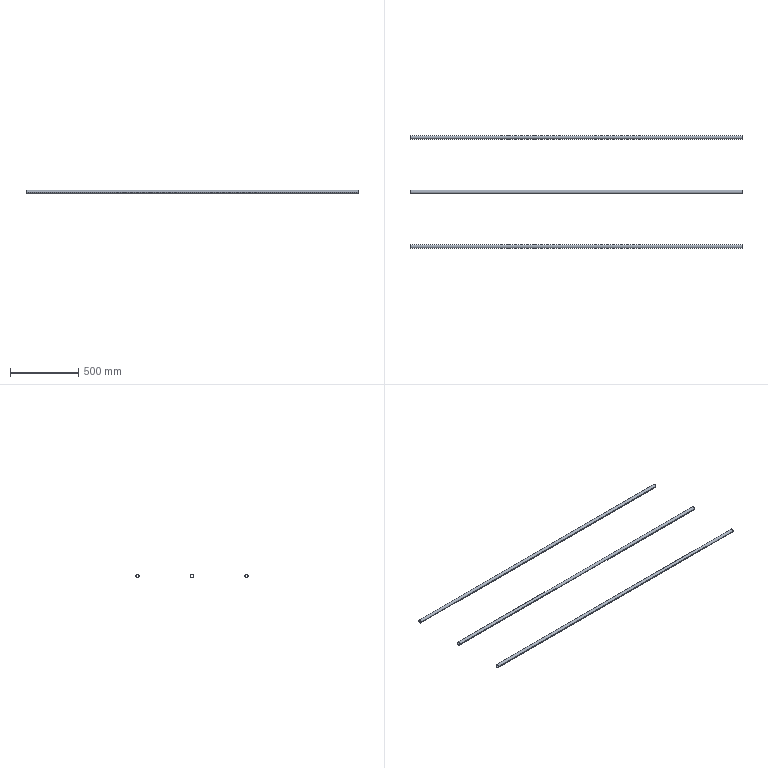Part | STEP file | 粉仓护栏栏杆4_Default<As Machined> | 3 solids | 18 faces | box 2430 x 825 x 25 mm | volume 807303 mm3 | cylinder 12 | plane 6 | commonest cylinder face diameters 22 x6 25 x6
STEP:
#1=CARTESIAN_POINT('',(0.,0.,0.));
#2=DIRECTION('',(0.,0.,1.));
#3=DIRECTION('',(1.,0.,0.));
#4=AXIS2_PLACEMENT_3D('',#1,#2,#3);
#5=CARTESIAN_POINT('',(1215.,812.5,0.));
#6=VERTEX_POINT('',#5);
#7=CARTESIAN_POINT('',(1215.,787.5,0.));
#8=VERTEX_POINT('',#7);
#9=CARTESIAN_POINT('',(1215.,800.,0.));
#10=DIRECTION('',(1.,0.,0.));
#11=DIRECTION('',(0.,1.,0.));
#12=AXIS2_PLACEMENT_3D('',#9,#10,#11);
#13=CIRCLE('',#12,12.5);
#14=CARTESIAN_POINT('',(1215.,800.,0.));
#15=DIRECTION('',(-1.,0.,0.));
#16=DIRECTION('',(0.,-1.,0.));
#17=AXIS2_PLACEMENT_3D('',#14,#15,#16);
#18=CYLINDRICAL_SURFACE('',#17,12.5);
#19=CARTESIAN_POINT('',(3.142,0.));
#20=DIRECTION('',(-1.,0.));
#21=VECTOR('',#20,1.);
#22=LINE('',#19,#21);
#23=(GEOMETRIC_REPRESENTATION_CONTEXT(2)PARAMETRIC_REPRESENTATION_CONTEXT()REPRESENTATION_CONTEXT('',''));
#24=DEFINITIONAL_REPRESENTATION('',(#22),#23);
#25=PCURVE('',#18,#24);
#26=CARTESIAN_POINT('',(1215.,800.,0.));
#27=DIRECTION('',(1.,0.,0.));
#28=DIRECTION('',(0.,1.,0.));
#29=AXIS2_PLACEMENT_3D('',#26,#27,#28);
#30=PLANE('',#29);
#31=CARTESIAN_POINT('',(0.,0.));
#32=DIRECTION('',(1.,0.));
#33=AXIS2_PLACEMENT_2D('',#31,#32);
#34=CIRCLE('',#33,12.5);
#35=(GEOMETRIC_REPRESENTATION_CONTEXT(2)PARAMETRIC_REPRESENTATION_CONTEXT()REPRESENTATION_CONTEXT('',''));
#36=DEFINITIONAL_REPRESENTATION('',(#34),#35);
#37=PCURVE('',#30,#36);
#38=SURFACE_CURVE('',#13,(#25,#37),.PCURVE_S1.);
#39=EDGE_CURVE('',#6,#8,#38,.T.);
#40=ORIENTED_EDGE('',*,*,#39,.F.);
#41=CARTESIAN_POINT('',(-1215.,812.5,0.));
#42=VERTEX_POINT('',#41);
#43=CARTESIAN_POINT('',(1215.,812.5,0.));
#44=DIRECTION('',(-1.,0.,0.));
#45=VECTOR('',#44,1.);
#46=LINE('',#43,#45);
#47=CARTESIAN_POINT('',(3.142,0.));
#48=DIRECTION('',(0.,1.));
#49=VECTOR('',#48,1.);
#50=LINE('',#47,#49);
#51=(GEOMETRIC_REPRESENTATION_CONTEXT(2)PARAMETRIC_REPRESENTATION_CONTEXT()REPRESENTATION_CONTEXT('',''));
#52=DEFINITIONAL_REPRESENTATION('',(#50),#51);
#53=PCURVE('',#18,#52);
#54=CARTESIAN_POINT('',(1215.,800.,0.));
#55=DIRECTION('',(-1.,0.,0.));
#56=DIRECTION('',(0.,-1.,0.));
#57=AXIS2_PLACEMENT_3D('',#54,#55,#56);
#58=CYLINDRICAL_SURFACE('',#57,12.5);
#59=CARTESIAN_POINT('',(3.142,0.));
#60=DIRECTION('',(0.,1.));
#61=VECTOR('',#60,1.);
#62=LINE('',#59,#61);
#63=(GEOMETRIC_REPRESENTATION_CONTEXT(2)PARAMETRIC_REPRESENTATION_CONTEXT()REPRESENTATION_CONTEXT('',''));
#64=DEFINITIONAL_REPRESENTATION('',(#62),#63);
#65=PCURVE('',#58,#64);
#66=SURFACE_CURVE('',#46,(#53,#65),.PCURVE_S1.);
#67=EDGE_CURVE('',#6,#42,#66,.T.);
#68=ORIENTED_EDGE('',*,*,#67,.T.);
#69=CARTESIAN_POINT('',(-1215.,787.5,0.));
#70=VERTEX_POINT('',#69);
#71=CARTESIAN_POINT('',(-1215.,800.,0.));
#72=DIRECTION('',(1.,0.,0.));
#73=DIRECTION('',(0.,1.,0.));
#74=AXIS2_PLACEMENT_3D('',#71,#72,#73);
#75=CIRCLE('',#74,12.5);
#76=CARTESIAN_POINT('',(3.142,2430.));
#77=DIRECTION('',(-1.,0.));
#78=VECTOR('',#77,1.);
#79=LINE('',#76,#78);
#80=(GEOMETRIC_REPRESENTATION_CONTEXT(2)PARAMETRIC_REPRESENTATION_CONTEXT()REPRESENTATION_CONTEXT('',''));
#81=DEFINITIONAL_REPRESENTATION('',(#79),#80);
#82=PCURVE('',#18,#81);
#83=CARTESIAN_POINT('',(-1215.,800.,0.));
#84=DIRECTION('',(1.,0.,0.));
#85=DIRECTION('',(0.,1.,0.));
#86=AXIS2_PLACEMENT_3D('',#83,#84,#85);
#87=PLANE('',#86);
#88=CARTESIAN_POINT('',(0.,0.));
#89=DIRECTION('',(1.,0.));
#90=AXIS2_PLACEMENT_2D('',#88,#89);
#91=CIRCLE('',#90,12.5);
#92=(GEOMETRIC_REPRESENTATION_CONTEXT(2)PARAMETRIC_REPRESENTATION_CONTEXT()REPRESENTATION_CONTEXT('',''));
#93=DEFINITIONAL_REPRESENTATION('',(#91),#92);
#94=PCURVE('',#87,#93);
#95=SURFACE_CURVE('',#75,(#82,#94),.PCURVE_S1.);
#96=EDGE_CURVE('',#42,#70,#95,.T.);
#97=ORIENTED_EDGE('',*,*,#96,.T.);
#98=CARTESIAN_POINT('',(1215.,787.5,0.));
#99=DIRECTION('',(-1.,0.,0.));
#100=VECTOR('',#99,1.);
#101=LINE('',#98,#100);
#102=CARTESIAN_POINT('',(0.,0.));
#103=DIRECTION('',(0.,1.));
#104=VECTOR('',#103,1.);
#105=LINE('',#102,#104);
#106=(GEOMETRIC_REPRESENTATION_CONTEXT(2)PARAMETRIC_REPRESENTATION_CONTEXT()REPRESENTATION_CONTEXT('',''));
#107=DEFINITIONAL_REPRESENTATION('',(#105),#106);
#108=PCURVE('',#18,#107);
#109=CARTESIAN_POINT('',(6.283,0.));
#110=DIRECTION('',(0.,1.));
#111=VECTOR('',#110,1.);
#112=LINE('',#109,#111);
#113=(GEOMETRIC_REPRESENTATION_CONTEXT(2)PARAMETRIC_REPRESENTATION_CONTEXT()REPRESENTATION_CONTEXT('',''));
#114=DEFINITIONAL_REPRESENTATION('',(#112),#113);
#115=PCURVE('',#58,#114);
#116=SURFACE_CURVE('',#101,(#108,#115),.PCURVE_S1.);
#117=EDGE_CURVE('',#8,#70,#116,.T.);
#118=ORIENTED_EDGE('',*,*,#117,.F.);
#119=EDGE_LOOP('',(#40,#68,#97,#118));
#120=FACE_BOUND('',#119,.T.);
#121=ADVANCED_FACE('',(#120),#18,.T.);
#122=CARTESIAN_POINT('',(1215.,789.,0.));
#123=VERTEX_POINT('',#122);
#124=CARTESIAN_POINT('',(-1215.,789.,0.));
#125=VERTEX_POINT('',#124);
#126=CARTESIAN_POINT('',(1215.,789.,0.));
#127=DIRECTION('',(-1.,0.,0.));
#128=VECTOR('',#127,1.);
#129=LINE('',#126,#128);
#130=CARTESIAN_POINT('',(1215.,800.,0.));
#131=DIRECTION('',(-1.,0.,0.));
#132=DIRECTION('',(0.,-1.,0.));
#133=AXIS2_PLACEMENT_3D('',#130,#131,#132);
#134=CYLINDRICAL_SURFACE('',#133,11.);
#135=CARTESIAN_POINT('',(6.283,0.));
#136=DIRECTION('',(0.,1.));
#137=VECTOR('',#136,1.);
#138=LINE('',#135,#137);
#139=(GEOMETRIC_REPRESENTATION_CONTEXT(2)PARAMETRIC_REPRESENTATION_CONTEXT()REPRESENTATION_CONTEXT('',''));
#140=DEFINITIONAL_REPRESENTATION('',(#138),#139);
#141=PCURVE('',#134,#140);
#142=CARTESIAN_POINT('',(1215.,800.,0.));
#143=DIRECTION('',(-1.,0.,0.));
#144=DIRECTION('',(0.,-1.,0.));
#145=AXIS2_PLACEMENT_3D('',#142,#143,#144);
#146=CYLINDRICAL_SURFACE('',#145,11.);
#147=CARTESIAN_POINT('',(0.,0.));
#148=DIRECTION('',(0.,1.));
#149=VECTOR('',#148,1.);
#150=LINE('',#147,#149);
#151=(GEOMETRIC_REPRESENTATION_CONTEXT(2)PARAMETRIC_REPRESENTATION_CONTEXT()REPRESENTATION_CONTEXT('',''));
#152=DEFINITIONAL_REPRESENTATION('',(#150),#151);
#153=PCURVE('',#146,#152);
#154=SURFACE_CURVE('',#129,(#141,#153),.PCURVE_S1.);
#155=EDGE_CURVE('',#123,#125,#154,.T.);
#156=ORIENTED_EDGE('',*,*,#155,.T.);
#157=CARTESIAN_POINT('',(-1215.,811.,0.));
#158=VERTEX_POINT('',#157);
#159=CARTESIAN_POINT('',(-1215.,800.,0.));
#160=DIRECTION('',(1.,0.,0.));
#161=DIRECTION('',(0.,1.,0.));
#162=AXIS2_PLACEMENT_3D('',#159,#160,#161);
#163=CIRCLE('',#162,11.);
#164=CARTESIAN_POINT('',(9.425,2430.));
#165=DIRECTION('',(-1.,0.));
#166=VECTOR('',#165,1.);
#167=LINE('',#164,#166);
#168=(GEOMETRIC_REPRESENTATION_CONTEXT(2)PARAMETRIC_REPRESENTATION_CONTEXT()REPRESENTATION_CONTEXT('',''));
#169=DEFINITIONAL_REPRESENTATION('',(#167),#168);
#170=PCURVE('',#134,#169);
#171=CARTESIAN_POINT('',(0.,0.));
#172=DIRECTION('',(1.,0.));
#173=AXIS2_PLACEMENT_2D('',#171,#172);
#174=CIRCLE('',#173,11.);
#175=(GEOMETRIC_REPRESENTATION_CONTEXT(2)PARAMETRIC_REPRESENTATION_CONTEXT()REPRESENTATION_CONTEXT('',''));
#176=DEFINITIONAL_REPRESENTATION('',(#174),#175);
#177=PCURVE('',#87,#176);
#178=SURFACE_CURVE('',#163,(#170,#177),.PCURVE_S1.);
#179=EDGE_CURVE('',#125,#158,#178,.T.);
#180=ORIENTED_EDGE('',*,*,#179,.T.);
#181=CARTESIAN_POINT('',(1215.,811.,0.));
#182=VERTEX_POINT('',#181);
#183=CARTESIAN_POINT('',(1215.,811.,0.));
#184=DIRECTION('',(-1.,0.,0.));
#185=VECTOR('',#184,1.);
#186=LINE('',#183,#185);
#187=CARTESIAN_POINT('',(3.142,0.));
#188=DIRECTION('',(0.,1.));
#189=VECTOR('',#188,1.);
#190=LINE('',#187,#189);
#191=(GEOMETRIC_REPRESENTATION_CONTEXT(2)PARAMETRIC_REPRESENTATION_CONTEXT()REPRESENTATION_CONTEXT('',''));
#192=DEFINITIONAL_REPRESENTATION('',(#190),#191);
#193=PCURVE('',#134,#192);
#194=CARTESIAN_POINT('',(3.142,0.));
#195=DIRECTION('',(0.,1.));
#196=VECTOR('',#195,1.);
#197=LINE('',#194,#196);
#198=(GEOMETRIC_REPRESENTATION_CONTEXT(2)PARAMETRIC_REPRESENTATION_CONTEXT()REPRESENTATION_CONTEXT('',''));
#199=DEFINITIONAL_REPRESENTATION('',(#197),#198);
#200=PCURVE('',#146,#199);
#201=SURFACE_CURVE('',#186,(#193,#200),.PCURVE_S1.);
#202=EDGE_CURVE('',#182,#158,#201,.T.);
#203=ORIENTED_EDGE('',*,*,#202,.F.);
#204=CARTESIAN_POINT('',(1215.,800.,0.));
#205=DIRECTION('',(1.,0.,0.));
#206=DIRECTION('',(0.,1.,0.));
#207=AXIS2_PLACEMENT_3D('',#204,#205,#206);
#208=CIRCLE('',#207,11.);
#209=CARTESIAN_POINT('',(9.425,0.));
#210=DIRECTION('',(-1.,0.));
#211=VECTOR('',#210,1.);
#212=LINE('',#209,#211);
#213=(GEOMETRIC_REPRESENTATION_CONTEXT(2)PARAMETRIC_REPRESENTATION_CONTEXT()REPRESENTATION_CONTEXT('',''));
#214=DEFINITIONAL_REPRESENTATION('',(#212),#213);
#215=PCURVE('',#134,#214);
#216=CARTESIAN_POINT('',(0.,0.));
#217=DIRECTION('',(1.,0.));
#218=AXIS2_PLACEMENT_2D('',#216,#217);
#219=CIRCLE('',#218,11.);
#220=(GEOMETRIC_REPRESENTATION_CONTEXT(2)PARAMETRIC_REPRESENTATION_CONTEXT()REPRESENTATION_CONTEXT('',''));
#221=DEFINITIONAL_REPRESENTATION('',(#219),#220);
#222=PCURVE('',#30,#221);
#223=SURFACE_CURVE('',#208,(#215,#222),.PCURVE_S1.);
#224=EDGE_CURVE('',#123,#182,#223,.T.);
#225=ORIENTED_EDGE('',*,*,#224,.F.);
#226=EDGE_LOOP('',(#156,#180,#203,#225));
#227=FACE_BOUND('',#226,.F.);
#228=ADVANCED_FACE('',(#227),#134,.F.);
#229=CARTESIAN_POINT('',(-1215.,800.,0.));
#230=DIRECTION('',(1.,0.,0.));
#231=DIRECTION('',(0.,1.,0.));
#232=AXIS2_PLACEMENT_3D('',#229,#230,#231);
#233=CIRCLE('',#232,11.);
#234=CARTESIAN_POINT('',(3.142,2430.));
#235=DIRECTION('',(-1.,0.));
#236=VECTOR('',#235,1.);
#237=LINE('',#234,#236);
#238=(GEOMETRIC_REPRESENTATION_CONTEXT(2)PARAMETRIC_REPRESENTATION_CONTEXT()REPRESENTATION_CONTEXT('',''));
#239=DEFINITIONAL_REPRESENTATION('',(#237),#238);
#240=PCURVE('',#146,#239);
#241=CARTESIAN_POINT('',(0.,0.));
#242=DIRECTION('',(1.,0.));
#243=AXIS2_PLACEMENT_2D('',#241,#242);
#244=CIRCLE('',#243,11.);
#245=(GEOMETRIC_REPRESENTATION_CONTEXT(2)PARAMETRIC_REPRESENTATION_CONTEXT()REPRESENTATION_CONTEXT('',''));
#246=DEFINITIONAL_REPRESENTATION('',(#244),#245);
#247=PCURVE('',#87,#246);
#248=SURFACE_CURVE('',#233,(#240,#247),.PCURVE_S1.);
#249=EDGE_CURVE('',#158,#125,#248,.T.);
#250=ORIENTED_EDGE('',*,*,#249,.T.);
#251=ORIENTED_EDGE('',*,*,#155,.F.);
#252=CARTESIAN_POINT('',(1215.,800.,0.));
#253=DIRECTION('',(1.,0.,0.));
#254=DIRECTION('',(0.,1.,0.));
#255=AXIS2_PLACEMENT_3D('',#252,#253,#254);
#256=CIRCLE('',#255,11.);
#257=CARTESIAN_POINT('',(3.142,0.));
#258=DIRECTION('',(-1.,0.));
#259=VECTOR('',#258,1.);
#260=LINE('',#257,#259);
#261=(GEOMETRIC_REPRESENTATION_CONTEXT(2)PARAMETRIC_REPRESENTATION_CONTEXT()REPRESENTATION_CONTEXT('',''));
#262=DEFINITIONAL_REPRESENTATION('',(#260),#261);
#263=PCURVE('',#146,#262);
#264=CARTESIAN_POINT('',(0.,0.));
#265=DIRECTION('',(1.,0.));
#266=AXIS2_PLACEMENT_2D('',#264,#265);
#267=CIRCLE('',#266,11.);
#268=(GEOMETRIC_REPRESENTATION_CONTEXT(2)PARAMETRIC_REPRESENTATION_CONTEXT()REPRESENTATION_CONTEXT('',''));
#269=DEFINITIONAL_REPRESENTATION('',(#267),#268);
#270=PCURVE('',#30,#269);
#271=SURFACE_CURVE('',#256,(#263,#270),.PCURVE_S1.);
#272=EDGE_CURVE('',#182,#123,#271,.T.);
#273=ORIENTED_EDGE('',*,*,#272,.F.);
#274=ORIENTED_EDGE('',*,*,#202,.T.);
#275=EDGE_LOOP('',(#250,#251,#273,#274));
#276=FACE_BOUND('',#275,.F.);
#277=ADVANCED_FACE('',(#276),#146,.F.);
#278=ORIENTED_EDGE('',*,*,#67,.F.);
#279=CARTESIAN_POINT('',(1215.,800.,0.));
#280=DIRECTION('',(1.,0.,0.));
#281=DIRECTION('',(0.,1.,0.));
#282=AXIS2_PLACEMENT_3D('',#279,#280,#281);
#283=CIRCLE('',#282,12.5);
#284=CARTESIAN_POINT('',(9.425,0.));
#285=DIRECTION('',(-1.,0.));
#286=VECTOR('',#285,1.);
#287=LINE('',#284,#286);
#288=(GEOMETRIC_REPRESENTATION_CONTEXT(2)PARAMETRIC_REPRESENTATION_CONTEXT()REPRESENTATION_CONTEXT('',''));
#289=DEFINITIONAL_REPRESENTATION('',(#287),#288);
#290=PCURVE('',#58,#289);
#291=CARTESIAN_POINT('',(0.,0.));
#292=DIRECTION('',(1.,0.));
#293=AXIS2_PLACEMENT_2D('',#291,#292);
#294=CIRCLE('',#293,12.5);
#295=(GEOMETRIC_REPRESENTATION_CONTEXT(2)PARAMETRIC_REPRESENTATION_CONTEXT()REPRESENTATION_CONTEXT('',''));
#296=DEFINITIONAL_REPRESENTATION('',(#294),#295);
#297=PCURVE('',#30,#296);
#298=SURFACE_CURVE('',#283,(#290,#297),.PCURVE_S1.);
#299=EDGE_CURVE('',#8,#6,#298,.T.);
#300=ORIENTED_EDGE('',*,*,#299,.F.);
#301=ORIENTED_EDGE('',*,*,#117,.T.);
#302=CARTESIAN_POINT('',(-1215.,800.,0.));
#303=DIRECTION('',(1.,0.,0.));
#304=DIRECTION('',(0.,1.,0.));
#305=AXIS2_PLACEMENT_3D('',#302,#303,#304);
#306=CIRCLE('',#305,12.5);
#307=CARTESIAN_POINT('',(9.425,2430.));
#308=DIRECTION('',(-1.,0.));
#309=VECTOR('',#308,1.);
#310=LINE('',#307,#309);
#311=(GEOMETRIC_REPRESENTATION_CONTEXT(2)PARAMETRIC_REPRESENTATION_CONTEXT()REPRESENTATION_CONTEXT('',''));
#312=DEFINITIONAL_REPRESENTATION('',(#310),#311);
#313=PCURVE('',#58,#312);
#314=CARTESIAN_POINT('',(0.,0.));
#315=DIRECTION('',(1.,0.));
#316=AXIS2_PLACEMENT_2D('',#314,#315);
#317=CIRCLE('',#316,12.5);
#318=(GEOMETRIC_REPRESENTATION_CONTEXT(2)PARAMETRIC_REPRESENTATION_CONTEXT()REPRESENTATION_CONTEXT('',''));
#319=DEFINITIONAL_REPRESENTATION('',(#317),#318);
#320=PCURVE('',#87,#319);
#321=SURFACE_CURVE('',#306,(#313,#320),.PCURVE_S1.);
#322=EDGE_CURVE('',#70,#42,#321,.T.);
#323=ORIENTED_EDGE('',*,*,#322,.T.);
#324=EDGE_LOOP('',(#278,#300,#301,#323));
#325=FACE_BOUND('',#324,.T.);
#326=ADVANCED_FACE('',(#325),#58,.T.);
#327=ORIENTED_EDGE('',*,*,#224,.F.);
#328=ORIENTED_EDGE('',*,*,#272,.F.);
#329=EDGE_LOOP('',(#327,#328));
#330=FACE_BOUND('',#329,.T.);
#331=ORIENTED_EDGE('',*,*,#299,.T.);
#332=ORIENTED_EDGE('',*,*,#39,.T.);
#333=EDGE_LOOP('',(#331,#332));
#334=FACE_BOUND('',#333,.T.);
#335=ADVANCED_FACE('',(#330,#334),#30,.T.);
#336=ORIENTED_EDGE('',*,*,#179,.T.);
#337=ORIENTED_EDGE('',*,*,#249,.T.);
#338=EDGE_LOOP('',(#336,#337));
#339=FACE_BOUND('',#338,.T.);
#340=ORIENTED_EDGE('',*,*,#322,.F.);
#341=ORIENTED_EDGE('',*,*,#96,.F.);
#342=EDGE_LOOP('',(#340,#341));
#343=FACE_BOUND('',#342,.T.);
#344=ADVANCED_FACE('',(#339,#343),#87,.F.);
#345=CLOSED_SHELL('',(#121,#228,#277,#326,#335,#344));
#346=MANIFOLD_SOLID_BREP('',#345);
#347=CARTESIAN_POINT('',(1215.,12.5,0.));
#348=VERTEX_POINT('',#347);
#349=CARTESIAN_POINT('',(1215.,-12.5,0.));
#350=VERTEX_POINT('',#349);
#351=CARTESIAN_POINT('',(1215.,0.,0.));
#352=DIRECTION('',(1.,0.,0.));
#353=DIRECTION('',(0.,1.,0.));
#354=AXIS2_PLACEMENT_3D('',#351,#352,#353);
#355=CIRCLE('',#354,12.5);
#356=CARTESIAN_POINT('',(1215.,0.,0.));
#357=DIRECTION('',(-1.,0.,0.));
#358=DIRECTION('',(0.,-1.,0.));
#359=AXIS2_PLACEMENT_3D('',#356,#357,#358);
#360=CYLINDRICAL_SURFACE('',#359,12.5);
#361=CARTESIAN_POINT('',(3.142,0.));
#362=DIRECTION('',(-1.,0.));
#363=VECTOR('',#362,1.);
#364=LINE('',#361,#363);
#365=(GEOMETRIC_REPRESENTATION_CONTEXT(2)PARAMETRIC_REPRESENTATION_CONTEXT()REPRESENTATION_CONTEXT('',''));
#366=DEFINITIONAL_REPRESENTATION('',(#364),#365);
#367=PCURVE('',#360,#366);
#368=CARTESIAN_POINT('',(1215.,0.,0.));
#369=DIRECTION('',(1.,0.,0.));
#370=DIRECTION('',(0.,1.,0.));
#371=AXIS2_PLACEMENT_3D('',#368,#369,#370);
#372=PLANE('',#371);
#373=CARTESIAN_POINT('',(0.,0.));
#374=DIRECTION('',(1.,0.));
#375=AXIS2_PLACEMENT_2D('',#373,#374);
#376=CIRCLE('',#375,12.5);
#377=(GEOMETRIC_REPRESENTATION_CONTEXT(2)PARAMETRIC_REPRESENTATION_CONTEXT()REPRESENTATION_CONTEXT('',''));
#378=DEFINITIONAL_REPRESENTATION('',(#376),#377);
#379=PCURVE('',#372,#378);
#380=SURFACE_CURVE('',#355,(#367,#379),.PCURVE_S1.);
#381=EDGE_CURVE('',#348,#350,#380,.T.);
#382=ORIENTED_EDGE('',*,*,#381,.F.);
#383=CARTESIAN_POINT('',(-1215.,12.5,0.));
#384=VERTEX_POINT('',#383);
#385=CARTESIAN_POINT('',(1215.,12.5,0.));
#386=DIRECTION('',(-1.,0.,0.));
#387=VECTOR('',#386,1.);
#388=LINE('',#385,#387);
#389=CARTESIAN_POINT('',(3.142,0.));
#390=DIRECTION('',(0.,1.));
#391=VECTOR('',#390,1.);
#392=LINE('',#389,#391);
#393=(GEOMETRIC_REPRESENTATION_CONTEXT(2)PARAMETRIC_REPRESENTATION_CONTEXT()REPRESENTATION_CONTEXT('',''));
#394=DEFINITIONAL_REPRESENTATION('',(#392),#393);
#395=PCURVE('',#360,#394);
#396=CARTESIAN_POINT('',(1215.,0.,0.));
#397=DIRECTION('',(-1.,0.,0.));
#398=DIRECTION('',(0.,-1.,0.));
#399=AXIS2_PLACEMENT_3D('',#396,#397,#398);
#400=CYLINDRICAL_SURFACE('',#399,12.5);
#401=CARTESIAN_POINT('',(3.142,0.));
#402=DIRECTION('',(0.,1.));
#403=VECTOR('',#402,1.);
#404=LINE('',#401,#403);
#405=(GEOMETRIC_REPRESENTATION_CONTEXT(2)PARAMETRIC_REPRESENTATION_CONTEXT()REPRESENTATION_CONTEXT('',''));
#406=DEFINITIONAL_REPRESENTATION('',(#404),#405);
#407=PCURVE('',#400,#406);
#408=SURFACE_CURVE('',#388,(#395,#407),.PCURVE_S1.);
#409=EDGE_CURVE('',#348,#384,#408,.T.);
#410=ORIENTED_EDGE('',*,*,#409,.T.);
#411=CARTESIAN_POINT('',(-1215.,-12.5,0.));
#412=VERTEX_POINT('',#411);
#413=CARTESIAN_POINT('',(-1215.,0.,0.));
#414=DIRECTION('',(1.,0.,0.));
#415=DIRECTION('',(0.,1.,0.));
#416=AXIS2_PLACEMENT_3D('',#413,#414,#415);
#417=CIRCLE('',#416,12.5);
#418=CARTESIAN_POINT('',(3.142,2430.));
#419=DIRECTION('',(-1.,0.));
#420=VECTOR('',#419,1.);
#421=LINE('',#418,#420);
#422=(GEOMETRIC_REPRESENTATION_CONTEXT(2)PARAMETRIC_REPRESENTATION_CONTEXT()REPRESENTATION_CONTEXT('',''));
#423=DEFINITIONAL_REPRESENTATION('',(#421),#422);
#424=PCURVE('',#360,#423);
#425=CARTESIAN_POINT('',(-1215.,0.,0.));
#426=DIRECTION('',(1.,0.,0.));
#427=DIRECTION('',(0.,1.,0.));
#428=AXIS2_PLACEMENT_3D('',#425,#426,#427);
#429=PLANE('',#428);
#430=CARTESIAN_POINT('',(0.,0.));
#431=DIRECTION('',(1.,0.));
#432=AXIS2_PLACEMENT_2D('',#430,#431);
#433=CIRCLE('',#432,12.5);
#434=(GEOMETRIC_REPRESENTATION_CONTEXT(2)PARAMETRIC_REPRESENTATION_CONTEXT()REPRESENTATION_CONTEXT('',''));
#435=DEFINITIONAL_REPRESENTATION('',(#433),#434);
#436=PCURVE('',#429,#435);
#437=SURFACE_CURVE('',#417,(#424,#436),.PCURVE_S1.);
#438=EDGE_CURVE('',#384,#412,#437,.T.);
#439=ORIENTED_EDGE('',*,*,#438,.T.);
#440=CARTESIAN_POINT('',(1215.,-12.5,0.));
#441=DIRECTION('',(-1.,0.,0.));
#442=VECTOR('',#441,1.);
#443=LINE('',#440,#442);
#444=CARTESIAN_POINT('',(0.,0.));
#445=DIRECTION('',(0.,1.));
#446=VECTOR('',#445,1.);
#447=LINE('',#444,#446);
#448=(GEOMETRIC_REPRESENTATION_CONTEXT(2)PARAMETRIC_REPRESENTATION_CONTEXT()REPRESENTATION_CONTEXT('',''));
#449=DEFINITIONAL_REPRESENTATION('',(#447),#448);
#450=PCURVE('',#360,#449);
#451=CARTESIAN_POINT('',(6.283,0.));
#452=DIRECTION('',(0.,1.));
#453=VECTOR('',#452,1.);
#454=LINE('',#451,#453);
#455=(GEOMETRIC_REPRESENTATION_CONTEXT(2)PARAMETRIC_REPRESENTATION_CONTEXT()REPRESENTATION_CONTEXT('',''));
#456=DEFINITIONAL_REPRESENTATION('',(#454),#455);
#457=PCURVE('',#400,#456);
#458=SURFACE_CURVE('',#443,(#450,#457),.PCURVE_S1.);
#459=EDGE_CURVE('',#350,#412,#458,.T.);
#460=ORIENTED_EDGE('',*,*,#459,.F.);
#461=EDGE_LOOP('',(#382,#410,#439,#460));
#462=FACE_BOUND('',#461,.T.);
#463=ADVANCED_FACE('',(#462),#360,.T.);
#464=CARTESIAN_POINT('',(1215.,-11.,0.));
#465=VERTEX_POINT('',#464);
#466=CARTESIAN_POINT('',(-1215.,-11.,0.));
#467=VERTEX_POINT('',#466);
#468=CARTESIAN_POINT('',(1215.,-11.,0.));
#469=DIRECTION('',(-1.,0.,0.));
#470=VECTOR('',#469,1.);
#471=LINE('',#468,#470);
#472=CARTESIAN_POINT('',(1215.,0.,0.));
#473=DIRECTION('',(-1.,0.,0.));
#474=DIRECTION('',(0.,-1.,0.));
#475=AXIS2_PLACEMENT_3D('',#472,#473,#474);
#476=CYLINDRICAL_SURFACE('',#475,11.);
#477=CARTESIAN_POINT('',(6.283,0.));
#478=DIRECTION('',(0.,1.));
#479=VECTOR('',#478,1.);
#480=LINE('',#477,#479);
#481=(GEOMETRIC_REPRESENTATION_CONTEXT(2)PARAMETRIC_REPRESENTATION_CONTEXT()REPRESENTATION_CONTEXT('',''));
#482=DEFINITIONAL_REPRESENTATION('',(#480),#481);
#483=PCURVE('',#476,#482);
#484=CARTESIAN_POINT('',(1215.,0.,0.));
#485=DIRECTION('',(-1.,0.,0.));
#486=DIRECTION('',(0.,-1.,0.));
#487=AXIS2_PLACEMENT_3D('',#484,#485,#486);
#488=CYLINDRICAL_SURFACE('',#487,11.);
#489=CARTESIAN_POINT('',(0.,0.));
#490=DIRECTION('',(0.,1.));
#491=VECTOR('',#490,1.);
#492=LINE('',#489,#491);
#493=(GEOMETRIC_REPRESENTATION_CONTEXT(2)PARAMETRIC_REPRESENTATION_CONTEXT()REPRESENTATION_CONTEXT('',''));
#494=DEFINITIONAL_REPRESENTATION('',(#492),#493);
#495=PCURVE('',#488,#494);
#496=SURFACE_CURVE('',#471,(#483,#495),.PCURVE_S1.);
#497=EDGE_CURVE('',#465,#467,#496,.T.);
#498=ORIENTED_EDGE('',*,*,#497,.T.);
#499=CARTESIAN_POINT('',(-1215.,11.,0.));
#500=VERTEX_POINT('',#499);
#501=CARTESIAN_POINT('',(-1215.,0.,0.));
#502=DIRECTION('',(1.,0.,0.));
#503=DIRECTION('',(0.,1.,0.));
#504=AXIS2_PLACEMENT_3D('',#501,#502,#503);
#505=CIRCLE('',#504,11.);
#506=CARTESIAN_POINT('',(9.425,2430.));
#507=DIRECTION('',(-1.,0.));
#508=VECTOR('',#507,1.);
#509=LINE('',#506,#508);
#510=(GEOMETRIC_REPRESENTATION_CONTEXT(2)PARAMETRIC_REPRESENTATION_CONTEXT()REPRESENTATION_CONTEXT('',''));
#511=DEFINITIONAL_REPRESENTATION('',(#509),#510);
#512=PCURVE('',#476,#511);
#513=CARTESIAN_POINT('',(0.,0.));
#514=DIRECTION('',(1.,0.));
#515=AXIS2_PLACEMENT_2D('',#513,#514);
#516=CIRCLE('',#515,11.);
#517=(GEOMETRIC_REPRESENTATION_CONTEXT(2)PARAMETRIC_REPRESENTATION_CONTEXT()REPRESENTATION_CONTEXT('',''));
#518=DEFINITIONAL_REPRESENTATION('',(#516),#517);
#519=PCURVE('',#429,#518);
#520=SURFACE_CURVE('',#505,(#512,#519),.PCURVE_S1.);
#521=EDGE_CURVE('',#467,#500,#520,.T.);
#522=ORIENTED_EDGE('',*,*,#521,.T.);
#523=CARTESIAN_POINT('',(1215.,11.,0.));
#524=VERTEX_POINT('',#523);
#525=CARTESIAN_POINT('',(1215.,11.,0.));
#526=DIRECTION('',(-1.,0.,0.));
#527=VECTOR('',#526,1.);
#528=LINE('',#525,#527);
#529=CARTESIAN_POINT('',(3.142,0.));
#530=DIRECTION('',(0.,1.));
#531=VECTOR('',#530,1.);
#532=LINE('',#529,#531);
#533=(GEOMETRIC_REPRESENTATION_CONTEXT(2)PARAMETRIC_REPRESENTATION_CONTEXT()REPRESENTATION_CONTEXT('',''));
#534=DEFINITIONAL_REPRESENTATION('',(#532),#533);
#535=PCURVE('',#476,#534);
#536=CARTESIAN_POINT('',(3.142,0.));
#537=DIRECTION('',(0.,1.));
#538=VECTOR('',#537,1.);
#539=LINE('',#536,#538);
#540=(GEOMETRIC_REPRESENTATION_CONTEXT(2)PARAMETRIC_REPRESENTATION_CONTEXT()REPRESENTATION_CONTEXT('',''));
#541=DEFINITIONAL_REPRESENTATION('',(#539),#540);
#542=PCURVE('',#488,#541);
#543=SURFACE_CURVE('',#528,(#535,#542),.PCURVE_S1.);
#544=EDGE_CURVE('',#524,#500,#543,.T.);
#545=ORIENTED_EDGE('',*,*,#544,.F.);
#546=CARTESIAN_POINT('',(1215.,0.,0.));
#547=DIRECTION('',(1.,0.,0.));
#548=DIRECTION('',(0.,1.,0.));
#549=AXIS2_PLACEMENT_3D('',#546,#547,#548);
#550=CIRCLE('',#549,11.);
#551=CARTESIAN_POINT('',(9.425,0.));
#552=DIRECTION('',(-1.,0.));
#553=VECTOR('',#552,1.);
#554=LINE('',#551,#553);
#555=(GEOMETRIC_REPRESENTATION_CONTEXT(2)PARAMETRIC_REPRESENTATION_CONTEXT()REPRESENTATION_CONTEXT('',''));
#556=DEFINITIONAL_REPRESENTATION('',(#554),#555);
#557=PCURVE('',#476,#556);
#558=CARTESIAN_POINT('',(0.,0.));
#559=DIRECTION('',(1.,0.));
#560=AXIS2_PLACEMENT_2D('',#558,#559);
#561=CIRCLE('',#560,11.);
#562=(GEOMETRIC_REPRESENTATION_CONTEXT(2)PARAMETRIC_REPRESENTATION_CONTEXT()REPRESENTATION_CONTEXT('',''));
#563=DEFINITIONAL_REPRESENTATION('',(#561),#562);
#564=PCURVE('',#372,#563);
#565=SURFACE_CURVE('',#550,(#557,#564),.PCURVE_S1.);
#566=EDGE_CURVE('',#465,#524,#565,.T.);
#567=ORIENTED_EDGE('',*,*,#566,.F.);
#568=EDGE_LOOP('',(#498,#522,#545,#567));
#569=FACE_BOUND('',#568,.F.);
#570=ADVANCED_FACE('',(#569),#476,.F.);
#571=CARTESIAN_POINT('',(-1215.,0.,0.));
#572=DIRECTION('',(1.,0.,0.));
#573=DIRECTION('',(0.,1.,0.));
#574=AXIS2_PLACEMENT_3D('',#571,#572,#573);
#575=CIRCLE('',#574,11.);
#576=CARTESIAN_POINT('',(3.142,2430.));
#577=DIRECTION('',(-1.,0.));
#578=VECTOR('',#577,1.);
#579=LINE('',#576,#578);
#580=(GEOMETRIC_REPRESENTATION_CONTEXT(2)PARAMETRIC_REPRESENTATION_CONTEXT()REPRESENTATION_CONTEXT('',''));
#581=DEFINITIONAL_REPRESENTATION('',(#579),#580);
#582=PCURVE('',#488,#581);
#583=CARTESIAN_POINT('',(0.,0.));
#584=DIRECTION('',(1.,0.));
#585=AXIS2_PLACEMENT_2D('',#583,#584);
#586=CIRCLE('',#585,11.);
#587=(GEOMETRIC_REPRESENTATION_CONTEXT(2)PARAMETRIC_REPRESENTATION_CONTEXT()REPRESENTATION_CONTEXT('',''));
#588=DEFINITIONAL_REPRESENTATION('',(#586),#587);
#589=PCURVE('',#429,#588);
#590=SURFACE_CURVE('',#575,(#582,#589),.PCURVE_S1.);
#591=EDGE_CURVE('',#500,#467,#590,.T.);
#592=ORIENTED_EDGE('',*,*,#591,.T.);
#593=ORIENTED_EDGE('',*,*,#497,.F.);
#594=CARTESIAN_POINT('',(1215.,0.,0.));
#595=DIRECTION('',(1.,0.,0.));
#596=DIRECTION('',(0.,1.,0.));
#597=AXIS2_PLACEMENT_3D('',#594,#595,#596);
#598=CIRCLE('',#597,11.);
#599=CARTESIAN_POINT('',(3.142,0.));
#600=DIRECTION('',(-1.,0.));
#601=VECTOR('',#600,1.);
#602=LINE('',#599,#601);
#603=(GEOMETRIC_REPRESENTATION_CONTEXT(2)PARAMETRIC_REPRESENTATION_CONTEXT()REPRESENTATION_CONTEXT('',''));
#604=DEFINITIONAL_REPRESENTATION('',(#602),#603);
#605=PCURVE('',#488,#604);
#606=CARTESIAN_POINT('',(0.,0.));
#607=DIRECTION('',(1.,0.));
#608=AXIS2_PLACEMENT_2D('',#606,#607);
#609=CIRCLE('',#608,11.);
#610=(GEOMETRIC_REPRESENTATION_CONTEXT(2)PARAMETRIC_REPRESENTATION_CONTEXT()REPRESENTATION_CONTEXT('',''));
#611=DEFINITIONAL_REPRESENTATION('',(#609),#610);
#612=PCURVE('',#372,#611);
#613=SURFACE_CURVE('',#598,(#605,#612),.PCURVE_S1.);
#614=EDGE_CURVE('',#524,#465,#613,.T.);
#615=ORIENTED_EDGE('',*,*,#614,.F.);
#616=ORIENTED_EDGE('',*,*,#544,.T.);
#617=EDGE_LOOP('',(#592,#593,#615,#616));
#618=FACE_BOUND('',#617,.F.);
#619=ADVANCED_FACE('',(#618),#488,.F.);
#620=ORIENTED_EDGE('',*,*,#409,.F.);
#621=CARTESIAN_POINT('',(1215.,0.,0.));
#622=DIRECTION('',(1.,0.,0.));
#623=DIRECTION('',(0.,1.,0.));
#624=AXIS2_PLACEMENT_3D('',#621,#622,#623);
#625=CIRCLE('',#624,12.5);
#626=CARTESIAN_POINT('',(9.425,0.));
#627=DIRECTION('',(-1.,0.));
#628=VECTOR('',#627,1.);
#629=LINE('',#626,#628);
#630=(GEOMETRIC_REPRESENTATION_CONTEXT(2)PARAMETRIC_REPRESENTATION_CONTEXT()REPRESENTATION_CONTEXT('',''));
#631=DEFINITIONAL_REPRESENTATION('',(#629),#630);
#632=PCURVE('',#400,#631);
#633=CARTESIAN_POINT('',(0.,0.));
#634=DIRECTION('',(1.,0.));
#635=AXIS2_PLACEMENT_2D('',#633,#634);
#636=CIRCLE('',#635,12.5);
#637=(GEOMETRIC_REPRESENTATION_CONTEXT(2)PARAMETRIC_REPRESENTATION_CONTEXT()REPRESENTATION_CONTEXT('',''));
#638=DEFINITIONAL_REPRESENTATION('',(#636),#637);
#639=PCURVE('',#372,#638);
#640=SURFACE_CURVE('',#625,(#632,#639),.PCURVE_S1.);
#641=EDGE_CURVE('',#350,#348,#640,.T.);
#642=ORIENTED_EDGE('',*,*,#641,.F.);
#643=ORIENTED_EDGE('',*,*,#459,.T.);
#644=CARTESIAN_POINT('',(-1215.,0.,0.));
#645=DIRECTION('',(1.,0.,0.));
#646=DIRECTION('',(0.,1.,0.));
#647=AXIS2_PLACEMENT_3D('',#644,#645,#646);
#648=CIRCLE('',#647,12.5);
#649=CARTESIAN_POINT('',(9.425,2430.));
#650=DIRECTION('',(-1.,0.));
#651=VECTOR('',#650,1.);
#652=LINE('',#649,#651);
#653=(GEOMETRIC_REPRESENTATION_CONTEXT(2)PARAMETRIC_REPRESENTATION_CONTEXT()REPRESENTATION_CONTEXT('',''));
#654=DEFINITIONAL_REPRESENTATION('',(#652),#653);
#655=PCURVE('',#400,#654);
#656=CARTESIAN_POINT('',(0.,0.));
#657=DIRECTION('',(1.,0.));
#658=AXIS2_PLACEMENT_2D('',#656,#657);
#659=CIRCLE('',#658,12.5);
#660=(GEOMETRIC_REPRESENTATION_CONTEXT(2)PARAMETRIC_REPRESENTATION_CONTEXT()REPRESENTATION_CONTEXT('',''));
#661=DEFINITIONAL_REPRESENTATION('',(#659),#660);
#662=PCURVE('',#429,#661);
#663=SURFACE_CURVE('',#648,(#655,#662),.PCURVE_S1.);
#664=EDGE_CURVE('',#412,#384,#663,.T.);
#665=ORIENTED_EDGE('',*,*,#664,.T.);
#666=EDGE_LOOP('',(#620,#642,#643,#665));
#667=FACE_BOUND('',#666,.T.);
#668=ADVANCED_FACE('',(#667),#400,.T.);
#669=ORIENTED_EDGE('',*,*,#566,.F.);
#670=ORIENTED_EDGE('',*,*,#614,.F.);
#671=EDGE_LOOP('',(#669,#670));
#672=FACE_BOUND('',#671,.T.);
#673=ORIENTED_EDGE('',*,*,#641,.T.);
#674=ORIENTED_EDGE('',*,*,#381,.T.);
#675=EDGE_LOOP('',(#673,#674));
#676=FACE_BOUND('',#675,.T.);
#677=ADVANCED_FACE('',(#672,#676),#372,.T.);
#678=ORIENTED_EDGE('',*,*,#521,.T.);
#679=ORIENTED_EDGE('',*,*,#591,.T.);
#680=EDGE_LOOP('',(#678,#679));
#681=FACE_BOUND('',#680,.T.);
#682=ORIENTED_EDGE('',*,*,#664,.F.);
#683=ORIENTED_EDGE('',*,*,#438,.F.);
#684=EDGE_LOOP('',(#682,#683));
#685=FACE_BOUND('',#684,.T.);
#686=ADVANCED_FACE('',(#681,#685),#429,.F.);
#687=CLOSED_SHELL('',(#463,#570,#619,#668,#677,#686));
#688=MANIFOLD_SOLID_BREP('',#687);
#689=CARTESIAN_POINT('',(1215.,412.5,0.));
#690=VERTEX_POINT('',#689);
#691=CARTESIAN_POINT('',(1215.,387.5,0.));
#692=VERTEX_POINT('',#691);
#693=CARTESIAN_POINT('',(1215.,400.,0.));
#694=DIRECTION('',(1.,0.,0.));
#695=DIRECTION('',(0.,1.,0.));
#696=AXIS2_PLACEMENT_3D('',#693,#694,#695);
#697=CIRCLE('',#696,12.5);
#698=CARTESIAN_POINT('',(1215.,400.,0.));
#699=DIRECTION('',(-1.,0.,0.));
#700=DIRECTION('',(0.,-1.,0.));
#701=AXIS2_PLACEMENT_3D('',#698,#699,#700);
#702=CYLINDRICAL_SURFACE('',#701,12.5);
#703=CARTESIAN_POINT('',(3.142,0.));
#704=DIRECTION('',(-1.,0.));
#705=VECTOR('',#704,1.);
#706=LINE('',#703,#705);
#707=(GEOMETRIC_REPRESENTATION_CONTEXT(2)PARAMETRIC_REPRESENTATION_CONTEXT()REPRESENTATION_CONTEXT('',''));
#708=DEFINITIONAL_REPRESENTATION('',(#706),#707);
#709=PCURVE('',#702,#708);
#710=CARTESIAN_POINT('',(1215.,400.,0.));
#711=DIRECTION('',(1.,0.,0.));
#712=DIRECTION('',(0.,1.,0.));
#713=AXIS2_PLACEMENT_3D('',#710,#711,#712);
#714=PLANE('',#713);
#715=CARTESIAN_POINT('',(0.,0.));
#716=DIRECTION('',(1.,0.));
#717=AXIS2_PLACEMENT_2D('',#715,#716);
#718=CIRCLE('',#717,12.5);
#719=(GEOMETRIC_REPRESENTATION_CONTEXT(2)PARAMETRIC_REPRESENTATION_CONTEXT()REPRESENTATION_CONTEXT('',''));
#720=DEFINITIONAL_REPRESENTATION('',(#718),#719);
#721=PCURVE('',#714,#720);
#722=SURFACE_CURVE('',#697,(#709,#721),.PCURVE_S1.);
#723=EDGE_CURVE('',#690,#692,#722,.T.);
#724=ORIENTED_EDGE('',*,*,#723,.F.);
#725=CARTESIAN_POINT('',(-1215.,412.5,0.));
#726=VERTEX_POINT('',#725);
#727=CARTESIAN_POINT('',(1215.,412.5,0.));
#728=DIRECTION('',(-1.,0.,0.));
#729=VECTOR('',#728,1.);
#730=LINE('',#727,#729);
#731=CARTESIAN_POINT('',(3.142,0.));
#732=DIRECTION('',(0.,1.));
#733=VECTOR('',#732,1.);
#734=LINE('',#731,#733);
#735=(GEOMETRIC_REPRESENTATION_CONTEXT(2)PARAMETRIC_REPRESENTATION_CONTEXT()REPRESENTATION_CONTEXT('',''));
#736=DEFINITIONAL_REPRESENTATION('',(#734),#735);
#737=PCURVE('',#702,#736);
#738=CARTESIAN_POINT('',(1215.,400.,0.));
#739=DIRECTION('',(-1.,0.,0.));
#740=DIRECTION('',(0.,-1.,0.));
#741=AXIS2_PLACEMENT_3D('',#738,#739,#740);
#742=CYLINDRICAL_SURFACE('',#741,12.5);
#743=CARTESIAN_POINT('',(3.142,0.));
#744=DIRECTION('',(0.,1.));
#745=VECTOR('',#744,1.);
#746=LINE('',#743,#745);
#747=(GEOMETRIC_REPRESENTATION_CONTEXT(2)PARAMETRIC_REPRESENTATION_CONTEXT()REPRESENTATION_CONTEXT('',''));
#748=DEFINITIONAL_REPRESENTATION('',(#746),#747);
#749=PCURVE('',#742,#748);
#750=SURFACE_CURVE('',#730,(#737,#749),.PCURVE_S1.);
#751=EDGE_CURVE('',#690,#726,#750,.T.);
#752=ORIENTED_EDGE('',*,*,#751,.T.);
#753=CARTESIAN_POINT('',(-1215.,387.5,0.));
#754=VERTEX_POINT('',#753);
#755=CARTESIAN_POINT('',(-1215.,400.,0.));
#756=DIRECTION('',(1.,0.,0.));
#757=DIRECTION('',(0.,1.,0.));
#758=AXIS2_PLACEMENT_3D('',#755,#756,#757);
#759=CIRCLE('',#758,12.5);
#760=CARTESIAN_POINT('',(3.142,2430.));
#761=DIRECTION('',(-1.,0.));
#762=VECTOR('',#761,1.);
#763=LINE('',#760,#762);
#764=(GEOMETRIC_REPRESENTATION_CONTEXT(2)PARAMETRIC_REPRESENTATION_CONTEXT()REPRESENTATION_CONTEXT('',''));
#765=DEFINITIONAL_REPRESENTATION('',(#763),#764);
#766=PCURVE('',#702,#765);
#767=CARTESIAN_POINT('',(-1215.,400.,0.));
#768=DIRECTION('',(1.,0.,0.));
#769=DIRECTION('',(0.,1.,0.));
#770=AXIS2_PLACEMENT_3D('',#767,#768,#769);
#771=PLANE('',#770);
#772=CARTESIAN_POINT('',(0.,0.));
#773=DIRECTION('',(1.,0.));
#774=AXIS2_PLACEMENT_2D('',#772,#773);
#775=CIRCLE('',#774,12.5);
#776=(GEOMETRIC_REPRESENTATION_CONTEXT(2)PARAMETRIC_REPRESENTATION_CONTEXT()REPRESENTATION_CONTEXT('',''));
#777=DEFINITIONAL_REPRESENTATION('',(#775),#776);
#778=PCURVE('',#771,#777);
#779=SURFACE_CURVE('',#759,(#766,#778),.PCURVE_S1.);
#780=EDGE_CURVE('',#726,#754,#779,.T.);
#781=ORIENTED_EDGE('',*,*,#780,.T.);
#782=CARTESIAN_POINT('',(1215.,387.5,0.));
#783=DIRECTION('',(-1.,0.,0.));
#784=VECTOR('',#783,1.);
#785=LINE('',#782,#784);
#786=CARTESIAN_POINT('',(0.,0.));
#787=DIRECTION('',(0.,1.));
#788=VECTOR('',#787,1.);
#789=LINE('',#786,#788);
#790=(GEOMETRIC_REPRESENTATION_CONTEXT(2)PARAMETRIC_REPRESENTATION_CONTEXT()REPRESENTATION_CONTEXT('',''));
#791=DEFINITIONAL_REPRESENTATION('',(#789),#790);
#792=PCURVE('',#702,#791);
#793=CARTESIAN_POINT('',(6.283,0.));
#794=DIRECTION('',(0.,1.));
#795=VECTOR('',#794,1.);
#796=LINE('',#793,#795);
#797=(GEOMETRIC_REPRESENTATION_CONTEXT(2)PARAMETRIC_REPRESENTATION_CONTEXT()REPRESENTATION_CONTEXT('',''));
#798=DEFINITIONAL_REPRESENTATION('',(#796),#797);
#799=PCURVE('',#742,#798);
#800=SURFACE_CURVE('',#785,(#792,#799),.PCURVE_S1.);
#801=EDGE_CURVE('',#692,#754,#800,.T.);
#802=ORIENTED_EDGE('',*,*,#801,.F.);
#803=EDGE_LOOP('',(#724,#752,#781,#802));
#804=FACE_BOUND('',#803,.T.);
#805=ADVANCED_FACE('',(#804),#702,.T.);
#806=CARTESIAN_POINT('',(1215.,389.,0.));
#807=VERTEX_POINT('',#806);
#808=CARTESIAN_POINT('',(-1215.,389.,0.));
#809=VERTEX_POINT('',#808);
#810=CARTESIAN_POINT('',(1215.,389.,0.));
#811=DIRECTION('',(-1.,0.,0.));
#812=VECTOR('',#811,1.);
#813=LINE('',#810,#812);
#814=CARTESIAN_POINT('',(1215.,400.,0.));
#815=DIRECTION('',(-1.,0.,0.));
#816=DIRECTION('',(0.,-1.,0.));
#817=AXIS2_PLACEMENT_3D('',#814,#815,#816);
#818=CYLINDRICAL_SURFACE('',#817,11.);
#819=CARTESIAN_POINT('',(6.283,0.));
#820=DIRECTION('',(0.,1.));
#821=VECTOR('',#820,1.);
#822=LINE('',#819,#821);
#823=(GEOMETRIC_REPRESENTATION_CONTEXT(2)PARAMETRIC_REPRESENTATION_CONTEXT()REPRESENTATION_CONTEXT('',''));
#824=DEFINITIONAL_REPRESENTATION('',(#822),#823);
#825=PCURVE('',#818,#824);
#826=CARTESIAN_POINT('',(1215.,400.,0.));
#827=DIRECTION('',(-1.,0.,0.));
#828=DIRECTION('',(0.,-1.,0.));
#829=AXIS2_PLACEMENT_3D('',#826,#827,#828);
#830=CYLINDRICAL_SURFACE('',#829,11.);
#831=CARTESIAN_POINT('',(0.,0.));
#832=DIRECTION('',(0.,1.));
#833=VECTOR('',#832,1.);
#834=LINE('',#831,#833);
#835=(GEOMETRIC_REPRESENTATION_CONTEXT(2)PARAMETRIC_REPRESENTATION_CONTEXT()REPRESENTATION_CONTEXT('',''));
#836=DEFINITIONAL_REPRESENTATION('',(#834),#835);
#837=PCURVE('',#830,#836);
#838=SURFACE_CURVE('',#813,(#825,#837),.PCURVE_S1.);
#839=EDGE_CURVE('',#807,#809,#838,.T.);
#840=ORIENTED_EDGE('',*,*,#839,.T.);
#841=CARTESIAN_POINT('',(-1215.,411.,0.));
#842=VERTEX_POINT('',#841);
#843=CARTESIAN_POINT('',(-1215.,400.,0.));
#844=DIRECTION('',(1.,0.,0.));
#845=DIRECTION('',(0.,1.,0.));
#846=AXIS2_PLACEMENT_3D('',#843,#844,#845);
#847=CIRCLE('',#846,11.);
#848=CARTESIAN_POINT('',(9.425,2430.));
#849=DIRECTION('',(-1.,0.));
#850=VECTOR('',#849,1.);
#851=LINE('',#848,#850);
#852=(GEOMETRIC_REPRESENTATION_CONTEXT(2)PARAMETRIC_REPRESENTATION_CONTEXT()REPRESENTATION_CONTEXT('',''));
#853=DEFINITIONAL_REPRESENTATION('',(#851),#852);
#854=PCURVE('',#818,#853);
#855=CARTESIAN_POINT('',(0.,0.));
#856=DIRECTION('',(1.,0.));
#857=AXIS2_PLACEMENT_2D('',#855,#856);
#858=CIRCLE('',#857,11.);
#859=(GEOMETRIC_REPRESENTATION_CONTEXT(2)PARAMETRIC_REPRESENTATION_CONTEXT()REPRESENTATION_CONTEXT('',''));
#860=DEFINITIONAL_REPRESENTATION('',(#858),#859);
#861=PCURVE('',#771,#860);
#862=SURFACE_CURVE('',#847,(#854,#861),.PCURVE_S1.);
#863=EDGE_CURVE('',#809,#842,#862,.T.);
#864=ORIENTED_EDGE('',*,*,#863,.T.);
#865=CARTESIAN_POINT('',(1215.,411.,0.));
#866=VERTEX_POINT('',#865);
#867=CARTESIAN_POINT('',(1215.,411.,0.));
#868=DIRECTION('',(-1.,0.,0.));
#869=VECTOR('',#868,1.);
#870=LINE('',#867,#869);
#871=CARTESIAN_POINT('',(3.142,0.));
#872=DIRECTION('',(0.,1.));
#873=VECTOR('',#872,1.);
#874=LINE('',#871,#873);
#875=(GEOMETRIC_REPRESENTATION_CONTEXT(2)PARAMETRIC_REPRESENTATION_CONTEXT()REPRESENTATION_CONTEXT('',''));
#876=DEFINITIONAL_REPRESENTATION('',(#874),#875);
#877=PCURVE('',#818,#876);
#878=CARTESIAN_POINT('',(3.142,0.));
#879=DIRECTION('',(0.,1.));
#880=VECTOR('',#879,1.);
#881=LINE('',#878,#880);
#882=(GEOMETRIC_REPRESENTATION_CONTEXT(2)PARAMETRIC_REPRESENTATION_CONTEXT()REPRESENTATION_CONTEXT('',''));
#883=DEFINITIONAL_REPRESENTATION('',(#881),#882);
#884=PCURVE('',#830,#883);
#885=SURFACE_CURVE('',#870,(#877,#884),.PCURVE_S1.);
#886=EDGE_CURVE('',#866,#842,#885,.T.);
#887=ORIENTED_EDGE('',*,*,#886,.F.);
#888=CARTESIAN_POINT('',(1215.,400.,0.));
#889=DIRECTION('',(1.,0.,0.));
#890=DIRECTION('',(0.,1.,0.));
#891=AXIS2_PLACEMENT_3D('',#888,#889,#890);
#892=CIRCLE('',#891,11.);
#893=CARTESIAN_POINT('',(9.425,0.));
#894=DIRECTION('',(-1.,0.));
#895=VECTOR('',#894,1.);
#896=LINE('',#893,#895);
#897=(GEOMETRIC_REPRESENTATION_CONTEXT(2)PARAMETRIC_REPRESENTATION_CONTEXT()REPRESENTATION_CONTEXT('',''));
#898=DEFINITIONAL_REPRESENTATION('',(#896),#897);
#899=PCURVE('',#818,#898);
#900=CARTESIAN_POINT('',(0.,0.));
#901=DIRECTION('',(1.,0.));
#902=AXIS2_PLACEMENT_2D('',#900,#901);
#903=CIRCLE('',#902,11.);
#904=(GEOMETRIC_REPRESENTATION_CONTEXT(2)PARAMETRIC_REPRESENTATION_CONTEXT()REPRESENTATION_CONTEXT('',''));
#905=DEFINITIONAL_REPRESENTATION('',(#903),#904);
#906=PCURVE('',#714,#905);
#907=SURFACE_CURVE('',#892,(#899,#906),.PCURVE_S1.);
#908=EDGE_CURVE('',#807,#866,#907,.T.);
#909=ORIENTED_EDGE('',*,*,#908,.F.);
#910=EDGE_LOOP('',(#840,#864,#887,#909));
#911=FACE_BOUND('',#910,.F.);
#912=ADVANCED_FACE('',(#911),#818,.F.);
#913=CARTESIAN_POINT('',(-1215.,400.,0.));
#914=DIRECTION('',(1.,0.,0.));
#915=DIRECTION('',(0.,1.,0.));
#916=AXIS2_PLACEMENT_3D('',#913,#914,#915);
#917=CIRCLE('',#916,11.);
#918=CARTESIAN_POINT('',(3.142,2430.));
#919=DIRECTION('',(-1.,0.));
#920=VECTOR('',#919,1.);
#921=LINE('',#918,#920);
#922=(GEOMETRIC_REPRESENTATION_CONTEXT(2)PARAMETRIC_REPRESENTATION_CONTEXT()REPRESENTATION_CONTEXT('',''));
#923=DEFINITIONAL_REPRESENTATION('',(#921),#922);
#924=PCURVE('',#830,#923);
#925=CARTESIAN_POINT('',(0.,0.));
#926=DIRECTION('',(1.,0.));
#927=AXIS2_PLACEMENT_2D('',#925,#926);
#928=CIRCLE('',#927,11.);
#929=(GEOMETRIC_REPRESENTATION_CONTEXT(2)PARAMETRIC_REPRESENTATION_CONTEXT()REPRESENTATION_CONTEXT('',''));
#930=DEFINITIONAL_REPRESENTATION('',(#928),#929);
#931=PCURVE('',#771,#930);
#932=SURFACE_CURVE('',#917,(#924,#931),.PCURVE_S1.);
#933=EDGE_CURVE('',#842,#809,#932,.T.);
#934=ORIENTED_EDGE('',*,*,#933,.T.);
#935=ORIENTED_EDGE('',*,*,#839,.F.);
#936=CARTESIAN_POINT('',(1215.,400.,0.));
#937=DIRECTION('',(1.,0.,0.));
#938=DIRECTION('',(0.,1.,0.));
#939=AXIS2_PLACEMENT_3D('',#936,#937,#938);
#940=CIRCLE('',#939,11.);
#941=CARTESIAN_POINT('',(3.142,0.));
#942=DIRECTION('',(-1.,0.));
#943=VECTOR('',#942,1.);
#944=LINE('',#941,#943);
#945=(GEOMETRIC_REPRESENTATION_CONTEXT(2)PARAMETRIC_REPRESENTATION_CONTEXT()REPRESENTATION_CONTEXT('',''));
#946=DEFINITIONAL_REPRESENTATION('',(#944),#945);
#947=PCURVE('',#830,#946);
#948=CARTESIAN_POINT('',(0.,0.));
#949=DIRECTION('',(1.,0.));
#950=AXIS2_PLACEMENT_2D('',#948,#949);
#951=CIRCLE('',#950,11.);
#952=(GEOMETRIC_REPRESENTATION_CONTEXT(2)PARAMETRIC_REPRESENTATION_CONTEXT()REPRESENTATION_CONTEXT('',''));
#953=DEFINITIONAL_REPRESENTATION('',(#951),#952);
#954=PCURVE('',#714,#953);
#955=SURFACE_CURVE('',#940,(#947,#954),.PCURVE_S1.);
#956=EDGE_CURVE('',#866,#807,#955,.T.);
#957=ORIENTED_EDGE('',*,*,#956,.F.);
#958=ORIENTED_EDGE('',*,*,#886,.T.);
#959=EDGE_LOOP('',(#934,#935,#957,#958));
#960=FACE_BOUND('',#959,.F.);
#961=ADVANCED_FACE('',(#960),#830,.F.);
#962=ORIENTED_EDGE('',*,*,#751,.F.);
#963=CARTESIAN_POINT('',(1215.,400.,0.));
#964=DIRECTION('',(1.,0.,0.));
#965=DIRECTION('',(0.,1.,0.));
#966=AXIS2_PLACEMENT_3D('',#963,#964,#965);
#967=CIRCLE('',#966,12.5);
#968=CARTESIAN_POINT('',(9.425,0.));
#969=DIRECTION('',(-1.,0.));
#970=VECTOR('',#969,1.);
#971=LINE('',#968,#970);
#972=(GEOMETRIC_REPRESENTATION_CONTEXT(2)PARAMETRIC_REPRESENTATION_CONTEXT()REPRESENTATION_CONTEXT('',''));
#973=DEFINITIONAL_REPRESENTATION('',(#971),#972);
#974=PCURVE('',#742,#973);
#975=CARTESIAN_POINT('',(0.,0.));
#976=DIRECTION('',(1.,0.));
#977=AXIS2_PLACEMENT_2D('',#975,#976);
#978=CIRCLE('',#977,12.5);
#979=(GEOMETRIC_REPRESENTATION_CONTEXT(2)PARAMETRIC_REPRESENTATION_CONTEXT()REPRESENTATION_CONTEXT('',''));
#980=DEFINITIONAL_REPRESENTATION('',(#978),#979);
#981=PCURVE('',#714,#980);
#982=SURFACE_CURVE('',#967,(#974,#981),.PCURVE_S1.);
#983=EDGE_CURVE('',#692,#690,#982,.T.);
#984=ORIENTED_EDGE('',*,*,#983,.F.);
#985=ORIENTED_EDGE('',*,*,#801,.T.);
#986=CARTESIAN_POINT('',(-1215.,400.,0.));
#987=DIRECTION('',(1.,0.,0.));
#988=DIRECTION('',(0.,1.,0.));
#989=AXIS2_PLACEMENT_3D('',#986,#987,#988);
#990=CIRCLE('',#989,12.5);
#991=CARTESIAN_POINT('',(9.425,2430.));
#992=DIRECTION('',(-1.,0.));
#993=VECTOR('',#992,1.);
#994=LINE('',#991,#993);
#995=(GEOMETRIC_REPRESENTATION_CONTEXT(2)PARAMETRIC_REPRESENTATION_CONTEXT()REPRESENTATION_CONTEXT('',''));
#996=DEFINITIONAL_REPRESENTATION('',(#994),#995);
#997=PCURVE('',#742,#996);
#998=CARTESIAN_POINT('',(0.,0.));
#999=DIRECTION('',(1.,0.));
#1000=AXIS2_PLACEMENT_2D('',#998,#999);
#1001=CIRCLE('',#1000,12.5);
#1002=(GEOMETRIC_REPRESENTATION_CONTEXT(2)PARAMETRIC_REPRESENTATION_CONTEXT()REPRESENTATION_CONTEXT('',''));
#1003=DEFINITIONAL_REPRESENTATION('',(#1001),#1002);
#1004=PCURVE('',#771,#1003);
#1005=SURFACE_CURVE('',#990,(#997,#1004),.PCURVE_S1.);
#1006=EDGE_CURVE('',#754,#726,#1005,.T.);
#1007=ORIENTED_EDGE('',*,*,#1006,.T.);
#1008=EDGE_LOOP('',(#962,#984,#985,#1007));
#1009=FACE_BOUND('',#1008,.T.);
#1010=ADVANCED_FACE('',(#1009),#742,.T.);
#1011=ORIENTED_EDGE('',*,*,#908,.F.);
#1012=ORIENTED_EDGE('',*,*,#956,.F.);
#1013=EDGE_LOOP('',(#1011,#1012));
#1014=FACE_BOUND('',#1013,.T.);
#1015=ORIENTED_EDGE('',*,*,#983,.T.);
#1016=ORIENTED_EDGE('',*,*,#723,.T.);
#1017=EDGE_LOOP('',(#1015,#1016));
#1018=FACE_BOUND('',#1017,.T.);
#1019=ADVANCED_FACE('',(#1014,#1018),#714,.T.);
#1020=ORIENTED_EDGE('',*,*,#863,.T.);
#1021=ORIENTED_EDGE('',*,*,#933,.T.);
#1022=EDGE_LOOP('',(#1020,#1021));
#1023=FACE_BOUND('',#1022,.T.);
#1024=ORIENTED_EDGE('',*,*,#1006,.F.);
#1025=ORIENTED_EDGE('',*,*,#780,.F.);
#1026=EDGE_LOOP('',(#1024,#1025));
#1027=FACE_BOUND('',#1026,.T.);
#1028=ADVANCED_FACE('',(#1023,#1027),#771,.F.);
#1029=CLOSED_SHELL('',(#805,#912,#961,#1010,#1019,#1028));
#1030=MANIFOLD_SOLID_BREP('',#1029);
#1031=(LENGTH_UNIT()NAMED_UNIT(*)SI_UNIT(.MILLI.,.METRE.));
#1032=UNCERTAINTY_MEASURE_WITH_UNIT(LENGTH_MEASURE(0.0000001),#1031,'','');
#1033=(NAMED_UNIT(*)PLANE_ANGLE_UNIT()SI_UNIT($,.RADIAN.));
#1034=(NAMED_UNIT(*)SI_UNIT($,.STERADIAN.)SOLID_ANGLE_UNIT());
#1035=(GEOMETRIC_REPRESENTATION_CONTEXT(3)GLOBAL_UNCERTAINTY_ASSIGNED_CONTEXT((#1032))GLOBAL_UNIT_ASSIGNED_CONTEXT((#1031,#1033,#1034))REPRESENTATION_CONTEXT('',''));
#1036=SHAPE_REPRESENTATION('',(#4,#346,#688,#1030),#1035);